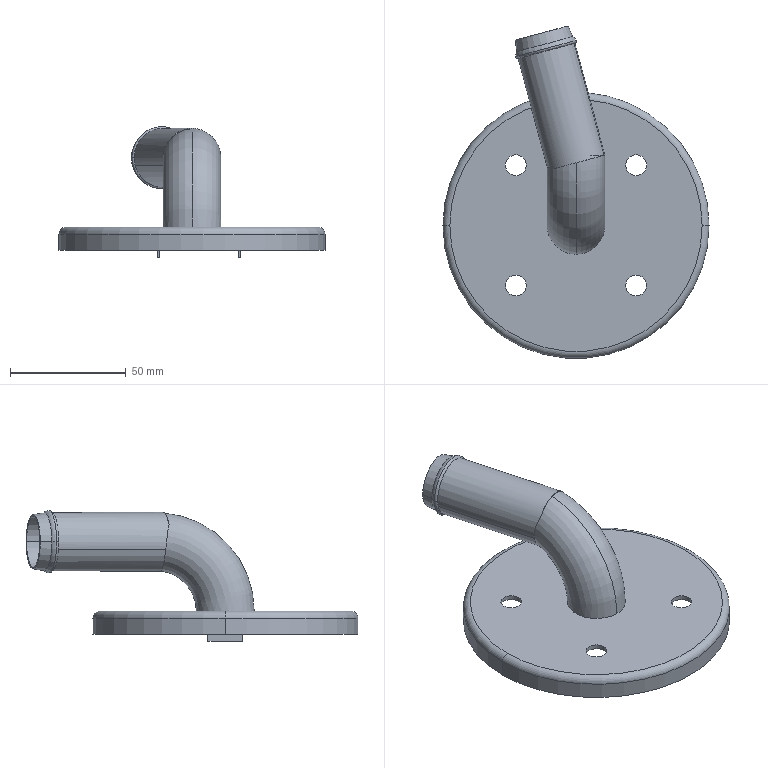Part | SolidWorks | features BaseBody 3 | 3 solids | 58 faces | box 115 x 143.577 x 56.488 mm | volume 37568 mm3 | plane 26 | cylinder 18 | torus 12 | cone 2 | commonest cylinder face diameters 9 x8 22 x4 25.38 x2 111 x2 115 x2